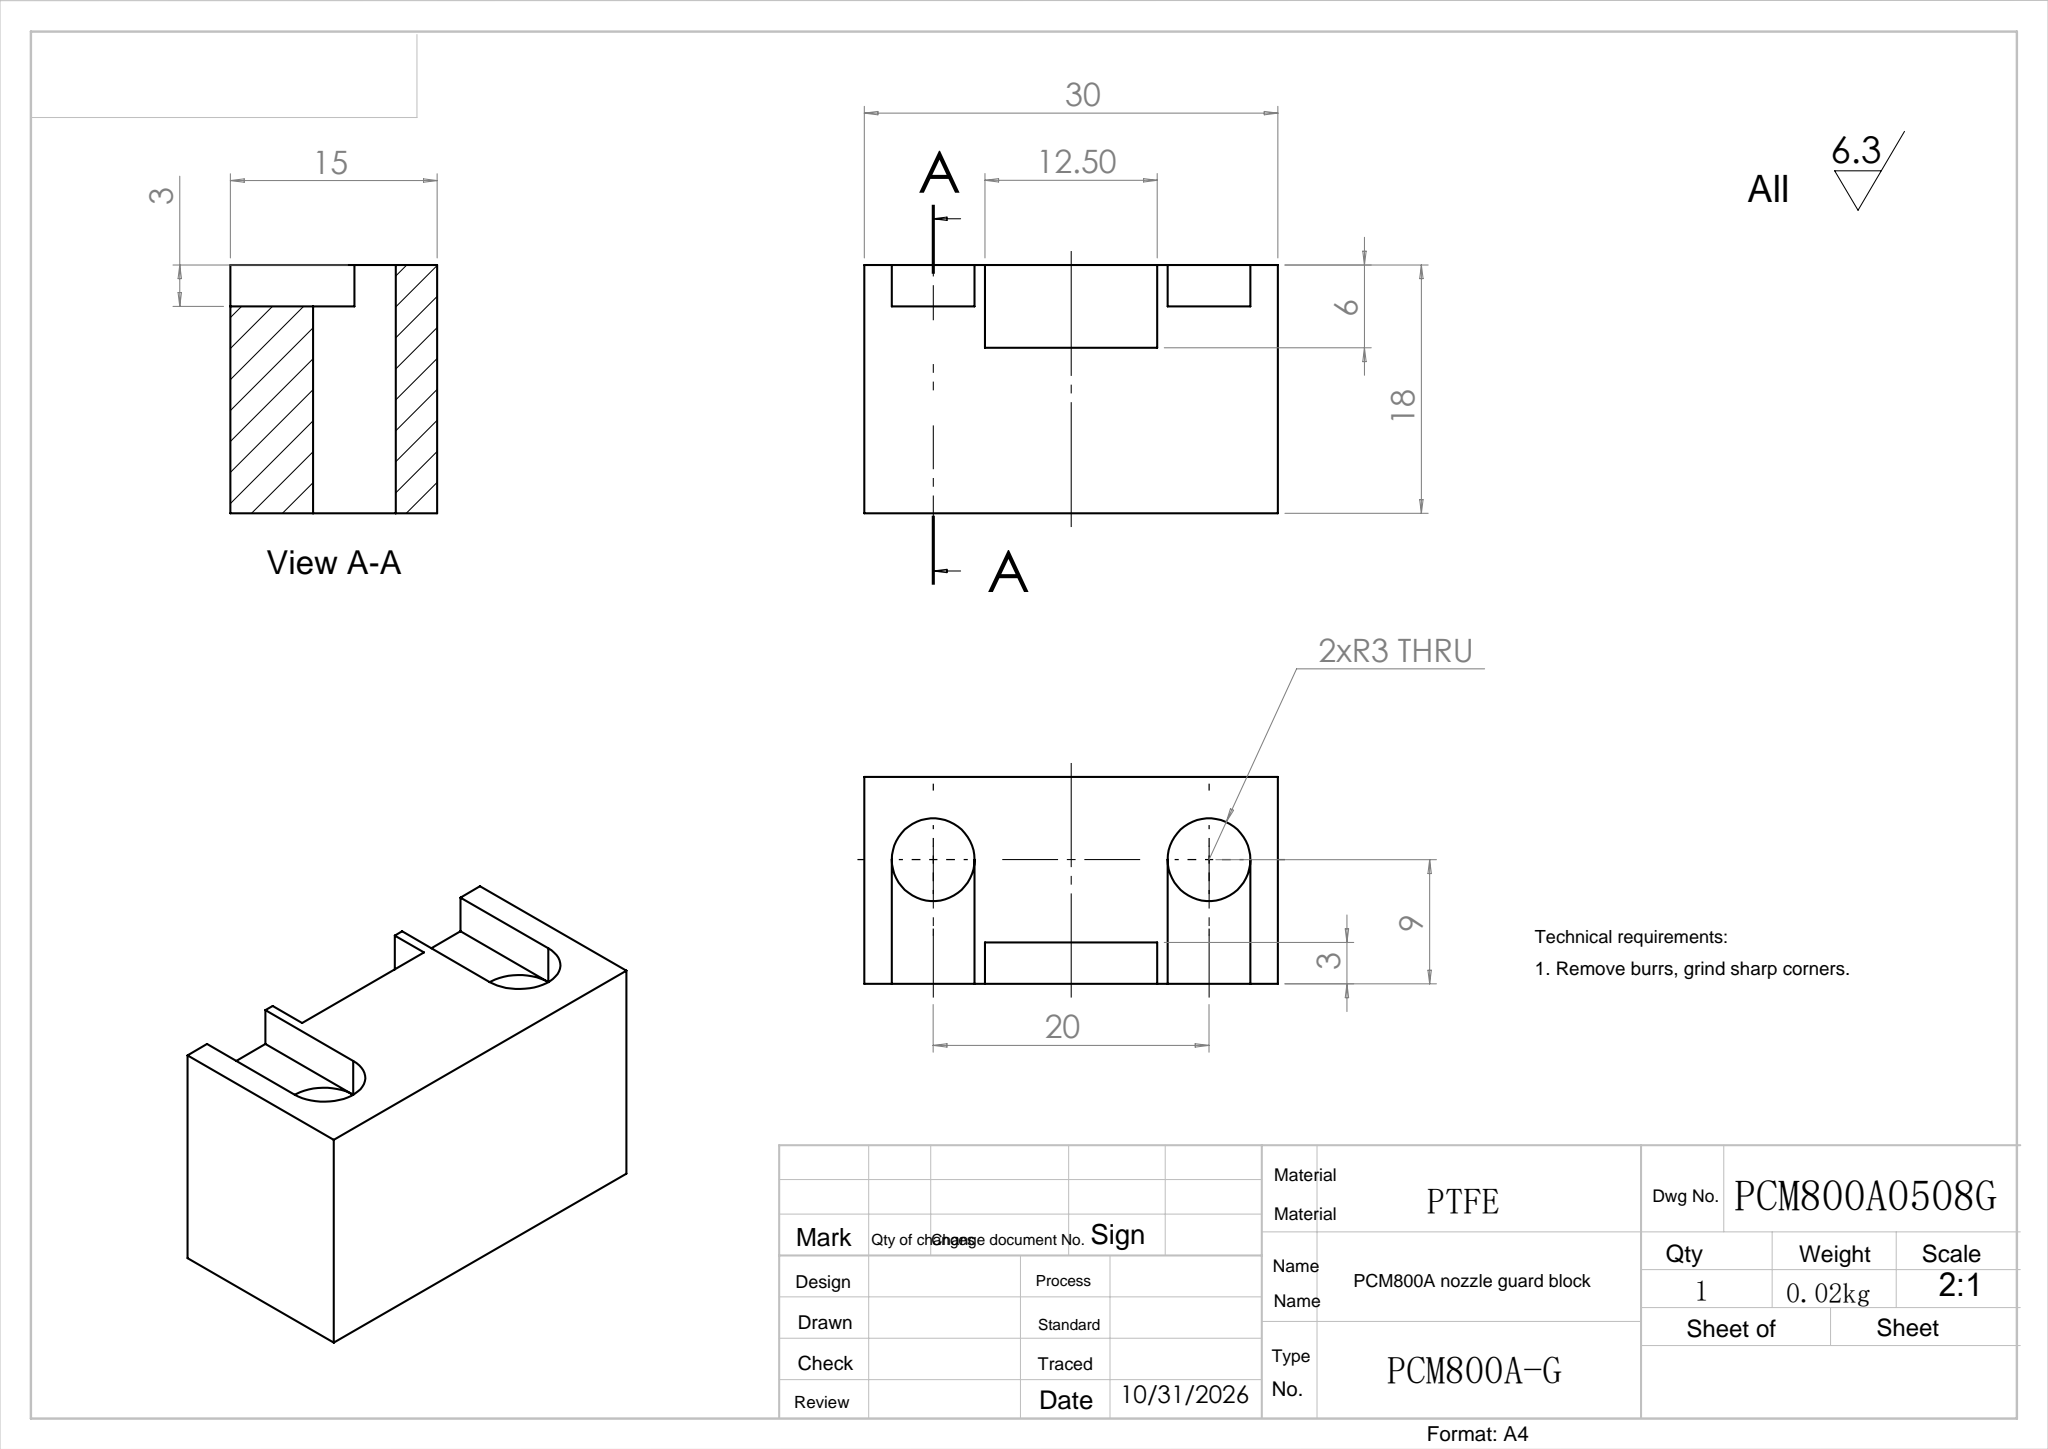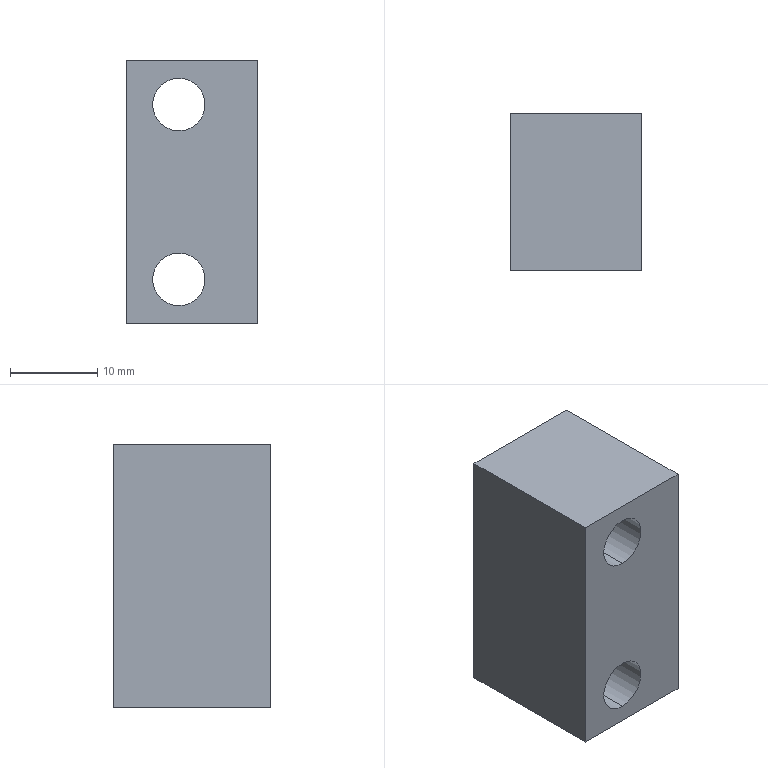Part | SolidWorks | features Cut 3, Extrusion 1, LPattern 1 | 1 solid | 20 faces | box 15 x 18 x 30 mm | volume 6618 mm3 | plane 16 | cylinder 4 | commonest cylinder face diameters 6 x4
STEP:
#1=CARTESIAN_POINT('',(6.,0.,22.));
#2=VERTEX_POINT('',#1);
#3=CARTESIAN_POINT('',(6.,0.,28.));
#4=VERTEX_POINT('',#3);
#5=CARTESIAN_POINT('',(6.,0.,25.));
#6=DIRECTION('',(0.,1.,0.));
#7=DIRECTION('',(0.,0.,1.));
#8=AXIS2_PLACEMENT_3D('',#5,#6,#7);
#9=CIRCLE('',#8,3.);
#10=EDGE_CURVE('',#2,#4,#9,.T.);
#11=ORIENTED_EDGE('',*,*,#10,.F.);
#12=CARTESIAN_POINT('',(6.,15.,22.));
#13=VERTEX_POINT('',#12);
#14=CARTESIAN_POINT('',(6.,0.,22.));
#15=DIRECTION('',(0.,1.,0.));
#16=VECTOR('',#15,1000.);
#17=LINE('',#14,#16);
#18=EDGE_CURVE('',#2,#13,#17,.T.);
#19=ORIENTED_EDGE('',*,*,#18,.T.);
#20=CARTESIAN_POINT('',(6.,18.,22.));
#21=VERTEX_POINT('',#20);
#22=CARTESIAN_POINT('',(6.,15.,22.));
#23=DIRECTION('',(0.,1.,0.));
#24=VECTOR('',#23,1000.);
#25=LINE('',#22,#24);
#26=EDGE_CURVE('',#13,#21,#25,.T.);
#27=ORIENTED_EDGE('',*,*,#26,.T.);
#28=CARTESIAN_POINT('',(6.,18.,28.));
#29=VERTEX_POINT('',#28);
#30=CARTESIAN_POINT('',(6.,18.,25.));
#31=DIRECTION('',(0.,1.,0.));
#32=DIRECTION('',(0.,0.,1.));
#33=AXIS2_PLACEMENT_3D('',#30,#31,#32);
#34=CIRCLE('',#33,3.);
#35=EDGE_CURVE('',#21,#29,#34,.T.);
#36=ORIENTED_EDGE('',*,*,#35,.T.);
#37=CARTESIAN_POINT('',(6.,15.,28.));
#38=VERTEX_POINT('',#37);
#39=CARTESIAN_POINT('',(6.,15.,28.));
#40=DIRECTION('',(0.,1.,0.));
#41=VECTOR('',#40,1000.);
#42=LINE('',#39,#41);
#43=EDGE_CURVE('',#38,#29,#42,.T.);
#44=ORIENTED_EDGE('',*,*,#43,.F.);
#45=CARTESIAN_POINT('',(6.,0.,28.));
#46=DIRECTION('',(0.,1.,0.));
#47=VECTOR('',#46,1000.);
#48=LINE('',#45,#47);
#49=EDGE_CURVE('',#4,#38,#48,.T.);
#50=ORIENTED_EDGE('',*,*,#49,.F.);
#51=EDGE_LOOP('',(#11,#19,#27,#36,#44,#50));
#52=FACE_OUTER_BOUND('',#51,.T.);
#53=CARTESIAN_POINT('',(6.,0.,25.));
#54=DIRECTION('',(0.,1.,0.));
#55=DIRECTION('',(0.,0.,1.));
#56=AXIS2_PLACEMENT_3D('',#53,#54,#55);
#57=CYLINDRICAL_SURFACE('',#56,3.);
#58=ADVANCED_FACE('',(#52),#57,.F.);
#59=CARTESIAN_POINT('',(6.,0.,2.));
#60=VERTEX_POINT('',#59);
#61=CARTESIAN_POINT('',(6.,0.,8.));
#62=VERTEX_POINT('',#61);
#63=CARTESIAN_POINT('',(6.,0.,5.));
#64=DIRECTION('',(0.,1.,0.));
#65=DIRECTION('',(0.,0.,1.));
#66=AXIS2_PLACEMENT_3D('',#63,#64,#65);
#67=CIRCLE('',#66,3.);
#68=EDGE_CURVE('',#60,#62,#67,.T.);
#69=ORIENTED_EDGE('',*,*,#68,.F.);
#70=CARTESIAN_POINT('',(6.,15.,2.));
#71=VERTEX_POINT('',#70);
#72=CARTESIAN_POINT('',(6.,0.,2.));
#73=DIRECTION('',(0.,1.,0.));
#74=VECTOR('',#73,1000.);
#75=LINE('',#72,#74);
#76=EDGE_CURVE('',#60,#71,#75,.T.);
#77=ORIENTED_EDGE('',*,*,#76,.T.);
#78=CARTESIAN_POINT('',(6.,18.,2.));
#79=VERTEX_POINT('',#78);
#80=CARTESIAN_POINT('',(6.,15.,2.));
#81=DIRECTION('',(0.,1.,0.));
#82=VECTOR('',#81,1000.);
#83=LINE('',#80,#82);
#84=EDGE_CURVE('',#71,#79,#83,.T.);
#85=ORIENTED_EDGE('',*,*,#84,.T.);
#86=CARTESIAN_POINT('',(6.,18.,8.));
#87=VERTEX_POINT('',#86);
#88=CARTESIAN_POINT('',(6.,18.,5.));
#89=DIRECTION('',(0.,1.,0.));
#90=DIRECTION('',(0.,0.,1.));
#91=AXIS2_PLACEMENT_3D('',#88,#89,#90);
#92=CIRCLE('',#91,3.);
#93=EDGE_CURVE('',#79,#87,#92,.T.);
#94=ORIENTED_EDGE('',*,*,#93,.T.);
#95=CARTESIAN_POINT('',(6.,15.,8.));
#96=VERTEX_POINT('',#95);
#97=CARTESIAN_POINT('',(6.,15.,8.));
#98=DIRECTION('',(0.,1.,0.));
#99=VECTOR('',#98,1000.);
#100=LINE('',#97,#99);
#101=EDGE_CURVE('',#96,#87,#100,.T.);
#102=ORIENTED_EDGE('',*,*,#101,.F.);
#103=CARTESIAN_POINT('',(6.,0.,8.));
#104=DIRECTION('',(0.,1.,0.));
#105=VECTOR('',#104,1000.);
#106=LINE('',#103,#105);
#107=EDGE_CURVE('',#62,#96,#106,.T.);
#108=ORIENTED_EDGE('',*,*,#107,.F.);
#109=EDGE_LOOP('',(#69,#77,#85,#94,#102,#108));
#110=FACE_OUTER_BOUND('',#109,.T.);
#111=CARTESIAN_POINT('',(6.,0.,5.));
#112=DIRECTION('',(0.,1.,0.));
#113=DIRECTION('',(0.,0.,1.));
#114=AXIS2_PLACEMENT_3D('',#111,#112,#113);
#115=CYLINDRICAL_SURFACE('',#114,3.);
#116=ADVANCED_FACE('',(#110),#115,.F.);
#117=CARTESIAN_POINT('',(15.,12.,21.25));
#118=VERTEX_POINT('',#117);
#119=CARTESIAN_POINT('',(15.,18.,21.25));
#120=VERTEX_POINT('',#119);
#121=CARTESIAN_POINT('',(15.,12.,21.25));
#122=DIRECTION('',(0.,1.,0.));
#123=VECTOR('',#122,1000.);
#124=LINE('',#121,#123);
#125=EDGE_CURVE('',#118,#120,#124,.T.);
#126=ORIENTED_EDGE('',*,*,#125,.T.);
#127=CARTESIAN_POINT('',(15.,18.,22.));
#128=VERTEX_POINT('',#127);
#129=CARTESIAN_POINT('',(15.,18.,30.));
#130=DIRECTION('',(0.,0.,-1.));
#131=VECTOR('',#130,1000.);
#132=LINE('',#129,#131);
#133=EDGE_CURVE('',#128,#120,#132,.T.);
#134=ORIENTED_EDGE('',*,*,#133,.F.);
#135=CARTESIAN_POINT('',(15.,15.,22.));
#136=VERTEX_POINT('',#135);
#137=CARTESIAN_POINT('',(15.,15.,22.));
#138=DIRECTION('',(0.,1.,0.));
#139=VECTOR('',#138,1000.);
#140=LINE('',#137,#139);
#141=EDGE_CURVE('',#136,#128,#140,.T.);
#142=ORIENTED_EDGE('',*,*,#141,.F.);
#143=CARTESIAN_POINT('',(15.,15.,28.));
#144=VERTEX_POINT('',#143);
#145=CARTESIAN_POINT('',(15.,15.,22.));
#146=DIRECTION('',(0.,0.,-1.));
#147=VECTOR('',#146,1000.);
#148=LINE('',#145,#147);
#149=EDGE_CURVE('',#144,#136,#148,.T.);
#150=ORIENTED_EDGE('',*,*,#149,.F.);
#151=CARTESIAN_POINT('',(15.,18.,28.));
#152=VERTEX_POINT('',#151);
#153=CARTESIAN_POINT('',(15.,15.,28.));
#154=DIRECTION('',(0.,1.,0.));
#155=VECTOR('',#154,1000.);
#156=LINE('',#153,#155);
#157=EDGE_CURVE('',#144,#152,#156,.T.);
#158=ORIENTED_EDGE('',*,*,#157,.T.);
#159=CARTESIAN_POINT('',(15.,18.,30.));
#160=VERTEX_POINT('',#159);
#161=CARTESIAN_POINT('',(15.,18.,30.));
#162=DIRECTION('',(0.,0.,-1.));
#163=VECTOR('',#162,1000.);
#164=LINE('',#161,#163);
#165=EDGE_CURVE('',#160,#152,#164,.T.);
#166=ORIENTED_EDGE('',*,*,#165,.F.);
#167=CARTESIAN_POINT('',(15.,0.,30.));
#168=VERTEX_POINT('',#167);
#169=CARTESIAN_POINT('',(15.,0.,30.));
#170=DIRECTION('',(0.,1.,0.));
#171=VECTOR('',#170,1000.);
#172=LINE('',#169,#171);
#173=EDGE_CURVE('',#168,#160,#172,.T.);
#174=ORIENTED_EDGE('',*,*,#173,.F.);
#175=CARTESIAN_POINT('',(15.,0.,0.));
#176=VERTEX_POINT('',#175);
#177=CARTESIAN_POINT('',(15.,0.,30.));
#178=DIRECTION('',(0.,0.,-1.));
#179=VECTOR('',#178,1000.);
#180=LINE('',#177,#179);
#181=EDGE_CURVE('',#168,#176,#180,.T.);
#182=ORIENTED_EDGE('',*,*,#181,.T.);
#183=CARTESIAN_POINT('',(15.,18.,0.));
#184=VERTEX_POINT('',#183);
#185=CARTESIAN_POINT('',(15.,0.,0.));
#186=DIRECTION('',(0.,1.,0.));
#187=VECTOR('',#186,1000.);
#188=LINE('',#185,#187);
#189=EDGE_CURVE('',#176,#184,#188,.T.);
#190=ORIENTED_EDGE('',*,*,#189,.T.);
#191=CARTESIAN_POINT('',(15.,18.,2.));
#192=VERTEX_POINT('',#191);
#193=CARTESIAN_POINT('',(15.,18.,30.));
#194=DIRECTION('',(0.,0.,-1.));
#195=VECTOR('',#194,1000.);
#196=LINE('',#193,#195);
#197=EDGE_CURVE('',#192,#184,#196,.T.);
#198=ORIENTED_EDGE('',*,*,#197,.F.);
#199=CARTESIAN_POINT('',(15.,15.,2.));
#200=VERTEX_POINT('',#199);
#201=CARTESIAN_POINT('',(15.,15.,2.));
#202=DIRECTION('',(0.,1.,0.));
#203=VECTOR('',#202,1000.);
#204=LINE('',#201,#203);
#205=EDGE_CURVE('',#200,#192,#204,.T.);
#206=ORIENTED_EDGE('',*,*,#205,.F.);
#207=CARTESIAN_POINT('',(15.,15.,8.));
#208=VERTEX_POINT('',#207);
#209=CARTESIAN_POINT('',(15.,15.,2.));
#210=DIRECTION('',(0.,0.,-1.));
#211=VECTOR('',#210,1000.);
#212=LINE('',#209,#211);
#213=EDGE_CURVE('',#208,#200,#212,.T.);
#214=ORIENTED_EDGE('',*,*,#213,.F.);
#215=CARTESIAN_POINT('',(15.,18.,8.));
#216=VERTEX_POINT('',#215);
#217=CARTESIAN_POINT('',(15.,15.,8.));
#218=DIRECTION('',(0.,1.,0.));
#219=VECTOR('',#218,1000.);
#220=LINE('',#217,#219);
#221=EDGE_CURVE('',#208,#216,#220,.T.);
#222=ORIENTED_EDGE('',*,*,#221,.T.);
#223=CARTESIAN_POINT('',(15.,18.,8.75));
#224=VERTEX_POINT('',#223);
#225=CARTESIAN_POINT('',(15.,18.,30.));
#226=DIRECTION('',(0.,0.,-1.));
#227=VECTOR('',#226,1000.);
#228=LINE('',#225,#227);
#229=EDGE_CURVE('',#224,#216,#228,.T.);
#230=ORIENTED_EDGE('',*,*,#229,.F.);
#231=CARTESIAN_POINT('',(15.,12.,8.75));
#232=VERTEX_POINT('',#231);
#233=CARTESIAN_POINT('',(15.,12.,8.75));
#234=DIRECTION('',(0.,-1.,0.));
#235=VECTOR('',#234,1000.);
#236=LINE('',#233,#235);
#237=EDGE_CURVE('',#224,#232,#236,.T.);
#238=ORIENTED_EDGE('',*,*,#237,.T.);
#239=CARTESIAN_POINT('',(15.,12.,21.25));
#240=DIRECTION('',(0.,0.,1.));
#241=VECTOR('',#240,1000.);
#242=LINE('',#239,#241);
#243=EDGE_CURVE('',#232,#118,#242,.T.);
#244=ORIENTED_EDGE('',*,*,#243,.T.);
#245=EDGE_LOOP('',(#126,#134,#142,#150,#158,#166,#174,#182,#190,#198,#206,#214,#222,#230,#238,#244));
#246=FACE_OUTER_BOUND('',#245,.T.);
#247=CARTESIAN_POINT('',(15.,0.,30.));
#248=DIRECTION('',(-1.,0.,0.));
#249=DIRECTION('',(0.,0.,1.));
#250=AXIS2_PLACEMENT_3D('',#247,#248,#249);
#251=PLANE('',#250);
#252=ADVANCED_FACE('',(#246),#251,.F.);
#253=CARTESIAN_POINT('',(12.,18.,21.25));
#254=VERTEX_POINT('',#253);
#255=CARTESIAN_POINT('',(12.,18.,21.25));
#256=DIRECTION('',(1.,0.,0.));
#257=VECTOR('',#256,1000.);
#258=LINE('',#255,#257);
#259=EDGE_CURVE('',#254,#120,#258,.T.);
#260=ORIENTED_EDGE('',*,*,#259,.F.);
#261=CARTESIAN_POINT('',(12.,18.,8.75));
#262=VERTEX_POINT('',#261);
#263=CARTESIAN_POINT('',(12.,18.,21.25));
#264=DIRECTION('',(0.,0.,-1.));
#265=VECTOR('',#264,1000.);
#266=LINE('',#263,#265);
#267=EDGE_CURVE('',#254,#262,#266,.T.);
#268=ORIENTED_EDGE('',*,*,#267,.T.);
#269=CARTESIAN_POINT('',(12.,18.,8.75));
#270=DIRECTION('',(1.,0.,0.));
#271=VECTOR('',#270,1000.);
#272=LINE('',#269,#271);
#273=EDGE_CURVE('',#262,#224,#272,.T.);
#274=ORIENTED_EDGE('',*,*,#273,.T.);
#275=ORIENTED_EDGE('',*,*,#229,.T.);
#276=CARTESIAN_POINT('',(15.,18.,8.));
#277=DIRECTION('',(1.,0.,0.));
#278=VECTOR('',#277,1000.);
#279=LINE('',#276,#278);
#280=EDGE_CURVE('',#87,#216,#279,.T.);
#281=ORIENTED_EDGE('',*,*,#280,.F.);
#282=ORIENTED_EDGE('',*,*,#93,.F.);
#283=CARTESIAN_POINT('',(15.,18.,2.));
#284=DIRECTION('',(-1.,0.,0.));
#285=VECTOR('',#284,1000.);
#286=LINE('',#283,#285);
#287=EDGE_CURVE('',#192,#79,#286,.T.);
#288=ORIENTED_EDGE('',*,*,#287,.F.);
#289=ORIENTED_EDGE('',*,*,#197,.T.);
#290=CARTESIAN_POINT('',(0.,18.,0.));
#291=VERTEX_POINT('',#290);
#292=CARTESIAN_POINT('',(0.,18.,0.));
#293=DIRECTION('',(-1.,0.,0.));
#294=VECTOR('',#293,1000.);
#295=LINE('',#292,#294);
#296=EDGE_CURVE('',#184,#291,#295,.T.);
#297=ORIENTED_EDGE('',*,*,#296,.T.);
#298=CARTESIAN_POINT('',(0.,18.,30.));
#299=VERTEX_POINT('',#298);
#300=CARTESIAN_POINT('',(0.,18.,30.));
#301=DIRECTION('',(0.,0.,-1.));
#302=VECTOR('',#301,1000.);
#303=LINE('',#300,#302);
#304=EDGE_CURVE('',#299,#291,#303,.T.);
#305=ORIENTED_EDGE('',*,*,#304,.F.);
#306=CARTESIAN_POINT('',(0.,18.,30.));
#307=DIRECTION('',(-1.,0.,0.));
#308=VECTOR('',#307,1000.);
#309=LINE('',#306,#308);
#310=EDGE_CURVE('',#160,#299,#309,.T.);
#311=ORIENTED_EDGE('',*,*,#310,.F.);
#312=ORIENTED_EDGE('',*,*,#165,.T.);
#313=CARTESIAN_POINT('',(15.,18.,28.));
#314=DIRECTION('',(1.,0.,0.));
#315=VECTOR('',#314,1000.);
#316=LINE('',#313,#315);
#317=EDGE_CURVE('',#29,#152,#316,.T.);
#318=ORIENTED_EDGE('',*,*,#317,.F.);
#319=ORIENTED_EDGE('',*,*,#35,.F.);
#320=CARTESIAN_POINT('',(15.,18.,22.));
#321=DIRECTION('',(-1.,0.,0.));
#322=VECTOR('',#321,1000.);
#323=LINE('',#320,#322);
#324=EDGE_CURVE('',#128,#21,#323,.T.);
#325=ORIENTED_EDGE('',*,*,#324,.F.);
#326=ORIENTED_EDGE('',*,*,#133,.T.);
#327=EDGE_LOOP('',(#260,#268,#274,#275,#281,#282,#288,#289,#297,#305,#311,#312,#318,#319,#325,#326));
#328=FACE_OUTER_BOUND('',#327,.T.);
#329=CARTESIAN_POINT('',(0.,18.,30.));
#330=DIRECTION('',(0.,-1.,0.));
#331=DIRECTION('',(0.,0.,-1.));
#332=AXIS2_PLACEMENT_3D('',#329,#330,#331);
#333=PLANE('',#332);
#334=ADVANCED_FACE('',(#328),#333,.F.);
#335=CARTESIAN_POINT('',(0.,0.,0.));
#336=VERTEX_POINT('',#335);
#337=CARTESIAN_POINT('',(0.,0.,0.));
#338=DIRECTION('',(0.,-1.,0.));
#339=VECTOR('',#338,1000.);
#340=LINE('',#337,#339);
#341=EDGE_CURVE('',#291,#336,#340,.T.);
#342=ORIENTED_EDGE('',*,*,#341,.T.);
#343=CARTESIAN_POINT('',(0.,0.,30.));
#344=VERTEX_POINT('',#343);
#345=CARTESIAN_POINT('',(0.,0.,30.));
#346=DIRECTION('',(0.,0.,-1.));
#347=VECTOR('',#346,1000.);
#348=LINE('',#345,#347);
#349=EDGE_CURVE('',#344,#336,#348,.T.);
#350=ORIENTED_EDGE('',*,*,#349,.F.);
#351=CARTESIAN_POINT('',(0.,0.,30.));
#352=DIRECTION('',(0.,-1.,0.));
#353=VECTOR('',#352,1000.);
#354=LINE('',#351,#353);
#355=EDGE_CURVE('',#299,#344,#354,.T.);
#356=ORIENTED_EDGE('',*,*,#355,.F.);
#357=ORIENTED_EDGE('',*,*,#304,.T.);
#358=EDGE_LOOP('',(#342,#350,#356,#357));
#359=FACE_OUTER_BOUND('',#358,.T.);
#360=CARTESIAN_POINT('',(0.,0.,30.));
#361=DIRECTION('',(1.,0.,0.));
#362=DIRECTION('',(0.,0.,-1.));
#363=AXIS2_PLACEMENT_3D('',#360,#361,#362);
#364=PLANE('',#363);
#365=ADVANCED_FACE('',(#359),#364,.F.);
#366=CARTESIAN_POINT('',(6.,0.,25.));
#367=DIRECTION('',(0.,1.,0.));
#368=DIRECTION('',(0.,0.,1.));
#369=AXIS2_PLACEMENT_3D('',#366,#367,#368);
#370=CIRCLE('',#369,3.);
#371=EDGE_CURVE('',#4,#2,#370,.T.);
#372=ORIENTED_EDGE('',*,*,#371,.T.);
#373=ORIENTED_EDGE('',*,*,#10,.T.);
#374=EDGE_LOOP('',(#372,#373));
#375=FACE_BOUND('',#374,.T.);
#376=CARTESIAN_POINT('',(6.,0.,5.));
#377=DIRECTION('',(0.,1.,0.));
#378=DIRECTION('',(0.,0.,1.));
#379=AXIS2_PLACEMENT_3D('',#376,#377,#378);
#380=CIRCLE('',#379,3.);
#381=EDGE_CURVE('',#62,#60,#380,.T.);
#382=ORIENTED_EDGE('',*,*,#381,.T.);
#383=ORIENTED_EDGE('',*,*,#68,.T.);
#384=EDGE_LOOP('',(#382,#383));
#385=FACE_BOUND('',#384,.T.);
#386=CARTESIAN_POINT('',(0.,0.,0.));
#387=DIRECTION('',(1.,0.,0.));
#388=VECTOR('',#387,1000.);
#389=LINE('',#386,#388);
#390=EDGE_CURVE('',#336,#176,#389,.T.);
#391=ORIENTED_EDGE('',*,*,#390,.T.);
#392=ORIENTED_EDGE('',*,*,#181,.F.);
#393=CARTESIAN_POINT('',(0.,0.,30.));
#394=DIRECTION('',(1.,0.,0.));
#395=VECTOR('',#394,1000.);
#396=LINE('',#393,#395);
#397=EDGE_CURVE('',#344,#168,#396,.T.);
#398=ORIENTED_EDGE('',*,*,#397,.F.);
#399=ORIENTED_EDGE('',*,*,#349,.T.);
#400=EDGE_LOOP('',(#391,#392,#398,#399));
#401=FACE_OUTER_BOUND('',#400,.T.);
#402=CARTESIAN_POINT('',(0.,0.,30.));
#403=DIRECTION('',(0.,1.,0.));
#404=DIRECTION('',(0.,0.,1.));
#405=AXIS2_PLACEMENT_3D('',#402,#403,#404);
#406=PLANE('',#405);
#407=ADVANCED_FACE('',(#375,#385,#401),#406,.F.);
#408=ORIENTED_EDGE('',*,*,#355,.T.);
#409=ORIENTED_EDGE('',*,*,#397,.T.);
#410=ORIENTED_EDGE('',*,*,#173,.T.);
#411=ORIENTED_EDGE('',*,*,#310,.T.);
#412=EDGE_LOOP('',(#408,#409,#410,#411));
#413=FACE_OUTER_BOUND('',#412,.T.);
#414=CARTESIAN_POINT('',(0.,18.,30.));
#415=DIRECTION('',(0.,0.,-1.));
#416=DIRECTION('',(-1.,0.,0.));
#417=AXIS2_PLACEMENT_3D('',#414,#415,#416);
#418=PLANE('',#417);
#419=ADVANCED_FACE('',(#413),#418,.F.);
#420=ORIENTED_EDGE('',*,*,#341,.F.);
#421=ORIENTED_EDGE('',*,*,#296,.F.);
#422=ORIENTED_EDGE('',*,*,#189,.F.);
#423=ORIENTED_EDGE('',*,*,#390,.F.);
#424=EDGE_LOOP('',(#420,#421,#422,#423));
#425=FACE_OUTER_BOUND('',#424,.T.);
#426=CARTESIAN_POINT('',(0.,18.,0.));
#427=DIRECTION('',(0.,0.,-1.));
#428=DIRECTION('',(-1.,0.,0.));
#429=AXIS2_PLACEMENT_3D('',#426,#427,#428);
#430=PLANE('',#429);
#431=ADVANCED_FACE('',(#425),#430,.T.);
#432=ORIENTED_EDGE('',*,*,#76,.F.);
#433=ORIENTED_EDGE('',*,*,#381,.F.);
#434=ORIENTED_EDGE('',*,*,#107,.T.);
#435=CARTESIAN_POINT('',(6.,15.,5.));
#436=DIRECTION('',(0.,-1.,0.));
#437=DIRECTION('',(0.,0.,1.));
#438=AXIS2_PLACEMENT_3D('',#435,#436,#437);
#439=CIRCLE('',#438,3.);
#440=EDGE_CURVE('',#71,#96,#439,.T.);
#441=ORIENTED_EDGE('',*,*,#440,.F.);
#442=EDGE_LOOP('',(#432,#433,#434,#441));
#443=FACE_OUTER_BOUND('',#442,.T.);
#444=CARTESIAN_POINT('',(6.,0.,5.));
#445=DIRECTION('',(0.,1.,0.));
#446=DIRECTION('',(0.,0.,1.));
#447=AXIS2_PLACEMENT_3D('',#444,#445,#446);
#448=CYLINDRICAL_SURFACE('',#447,3.);
#449=ADVANCED_FACE('',(#443),#448,.F.);
#450=ORIENTED_EDGE('',*,*,#440,.T.);
#451=CARTESIAN_POINT('',(15.,15.,8.));
#452=DIRECTION('',(1.,0.,0.));
#453=VECTOR('',#452,1000.);
#454=LINE('',#451,#453);
#455=EDGE_CURVE('',#96,#208,#454,.T.);
#456=ORIENTED_EDGE('',*,*,#455,.T.);
#457=ORIENTED_EDGE('',*,*,#213,.T.);
#458=CARTESIAN_POINT('',(15.,15.,2.));
#459=DIRECTION('',(-1.,0.,0.));
#460=VECTOR('',#459,1000.);
#461=LINE('',#458,#460);
#462=EDGE_CURVE('',#200,#71,#461,.T.);
#463=ORIENTED_EDGE('',*,*,#462,.T.);
#464=EDGE_LOOP('',(#450,#456,#457,#463));
#465=FACE_OUTER_BOUND('',#464,.T.);
#466=CARTESIAN_POINT('',(6.,15.,5.));
#467=DIRECTION('',(0.,1.,0.));
#468=DIRECTION('',(0.,0.,1.));
#469=AXIS2_PLACEMENT_3D('',#466,#467,#468);
#470=PLANE('',#469);
#471=ADVANCED_FACE('',(#465),#470,.T.);
#472=ORIENTED_EDGE('',*,*,#280,.T.);
#473=ORIENTED_EDGE('',*,*,#221,.F.);
#474=ORIENTED_EDGE('',*,*,#455,.F.);
#475=ORIENTED_EDGE('',*,*,#101,.T.);
#476=EDGE_LOOP('',(#472,#473,#474,#475));
#477=FACE_OUTER_BOUND('',#476,.T.);
#478=CARTESIAN_POINT('',(15.,15.,8.));
#479=DIRECTION('',(0.,0.,1.));
#480=DIRECTION('',(1.,0.,0.));
#481=AXIS2_PLACEMENT_3D('',#478,#479,#480);
#482=PLANE('',#481);
#483=ADVANCED_FACE('',(#477),#482,.F.);
#484=ORIENTED_EDGE('',*,*,#287,.T.);
#485=ORIENTED_EDGE('',*,*,#84,.F.);
#486=ORIENTED_EDGE('',*,*,#462,.F.);
#487=ORIENTED_EDGE('',*,*,#205,.T.);
#488=EDGE_LOOP('',(#484,#485,#486,#487));
#489=FACE_OUTER_BOUND('',#488,.T.);
#490=CARTESIAN_POINT('',(15.,15.,2.));
#491=DIRECTION('',(0.,0.,-1.));
#492=DIRECTION('',(-1.,0.,0.));
#493=AXIS2_PLACEMENT_3D('',#490,#491,#492);
#494=PLANE('',#493);
#495=ADVANCED_FACE('',(#489),#494,.F.);
#496=ORIENTED_EDGE('',*,*,#18,.F.);
#497=ORIENTED_EDGE('',*,*,#371,.F.);
#498=ORIENTED_EDGE('',*,*,#49,.T.);
#499=CARTESIAN_POINT('',(6.,15.,25.));
#500=DIRECTION('',(0.,-1.,0.));
#501=DIRECTION('',(0.,0.,1.));
#502=AXIS2_PLACEMENT_3D('',#499,#500,#501);
#503=CIRCLE('',#502,3.);
#504=EDGE_CURVE('',#13,#38,#503,.T.);
#505=ORIENTED_EDGE('',*,*,#504,.F.);
#506=EDGE_LOOP('',(#496,#497,#498,#505));
#507=FACE_OUTER_BOUND('',#506,.T.);
#508=CARTESIAN_POINT('',(6.,0.,25.));
#509=DIRECTION('',(0.,1.,0.));
#510=DIRECTION('',(0.,0.,1.));
#511=AXIS2_PLACEMENT_3D('',#508,#509,#510);
#512=CYLINDRICAL_SURFACE('',#511,3.);
#513=ADVANCED_FACE('',(#507),#512,.F.);
#514=ORIENTED_EDGE('',*,*,#504,.T.);
#515=CARTESIAN_POINT('',(15.,15.,28.));
#516=DIRECTION('',(1.,0.,0.));
#517=VECTOR('',#516,1000.);
#518=LINE('',#515,#517);
#519=EDGE_CURVE('',#38,#144,#518,.T.);
#520=ORIENTED_EDGE('',*,*,#519,.T.);
#521=ORIENTED_EDGE('',*,*,#149,.T.);
#522=CARTESIAN_POINT('',(15.,15.,22.));
#523=DIRECTION('',(-1.,0.,0.));
#524=VECTOR('',#523,1000.);
#525=LINE('',#522,#524);
#526=EDGE_CURVE('',#136,#13,#525,.T.);
#527=ORIENTED_EDGE('',*,*,#526,.T.);
#528=EDGE_LOOP('',(#514,#520,#521,#527));
#529=FACE_OUTER_BOUND('',#528,.T.);
#530=CARTESIAN_POINT('',(6.,15.,25.));
#531=DIRECTION('',(0.,1.,0.));
#532=DIRECTION('',(0.,0.,1.));
#533=AXIS2_PLACEMENT_3D('',#530,#531,#532);
#534=PLANE('',#533);
#535=ADVANCED_FACE('',(#529),#534,.T.);
#536=ORIENTED_EDGE('',*,*,#317,.T.);
#537=ORIENTED_EDGE('',*,*,#157,.F.);
#538=ORIENTED_EDGE('',*,*,#519,.F.);
#539=ORIENTED_EDGE('',*,*,#43,.T.);
#540=EDGE_LOOP('',(#536,#537,#538,#539));
#541=FACE_OUTER_BOUND('',#540,.T.);
#542=CARTESIAN_POINT('',(15.,15.,28.));
#543=DIRECTION('',(0.,0.,1.));
#544=DIRECTION('',(1.,0.,0.));
#545=AXIS2_PLACEMENT_3D('',#542,#543,#544);
#546=PLANE('',#545);
#547=ADVANCED_FACE('',(#541),#546,.F.);
#548=ORIENTED_EDGE('',*,*,#324,.T.);
#549=ORIENTED_EDGE('',*,*,#26,.F.);
#550=ORIENTED_EDGE('',*,*,#526,.F.);
#551=ORIENTED_EDGE('',*,*,#141,.T.);
#552=EDGE_LOOP('',(#548,#549,#550,#551));
#553=FACE_OUTER_BOUND('',#552,.T.);
#554=CARTESIAN_POINT('',(15.,15.,22.));
#555=DIRECTION('',(0.,0.,-1.));
#556=DIRECTION('',(-1.,0.,0.));
#557=AXIS2_PLACEMENT_3D('',#554,#555,#556);
#558=PLANE('',#557);
#559=ADVANCED_FACE('',(#553),#558,.F.);
#560=ORIENTED_EDGE('',*,*,#243,.F.);
#561=CARTESIAN_POINT('',(12.,12.,8.75));
#562=VERTEX_POINT('',#561);
#563=CARTESIAN_POINT('',(12.,12.,8.75));
#564=DIRECTION('',(1.,0.,0.));
#565=VECTOR('',#564,1000.);
#566=LINE('',#563,#565);
#567=EDGE_CURVE('',#562,#232,#566,.T.);
#568=ORIENTED_EDGE('',*,*,#567,.F.);
#569=CARTESIAN_POINT('',(12.,12.,21.25));
#570=VERTEX_POINT('',#569);
#571=CARTESIAN_POINT('',(12.,12.,21.25));
#572=DIRECTION('',(0.,0.,1.));
#573=VECTOR('',#572,1000.);
#574=LINE('',#571,#573);
#575=EDGE_CURVE('',#562,#570,#574,.T.);
#576=ORIENTED_EDGE('',*,*,#575,.T.);
#577=CARTESIAN_POINT('',(12.,12.,21.25));
#578=DIRECTION('',(1.,0.,0.));
#579=VECTOR('',#578,1000.);
#580=LINE('',#577,#579);
#581=EDGE_CURVE('',#570,#118,#580,.T.);
#582=ORIENTED_EDGE('',*,*,#581,.T.);
#583=EDGE_LOOP('',(#560,#568,#576,#582));
#584=FACE_OUTER_BOUND('',#583,.T.);
#585=CARTESIAN_POINT('',(12.,12.,21.25));
#586=DIRECTION('',(0.,1.,0.));
#587=DIRECTION('',(0.,0.,1.));
#588=AXIS2_PLACEMENT_3D('',#585,#586,#587);
#589=PLANE('',#588);
#590=ADVANCED_FACE('',(#584),#589,.T.);
#591=ORIENTED_EDGE('',*,*,#125,.F.);
#592=ORIENTED_EDGE('',*,*,#581,.F.);
#593=CARTESIAN_POINT('',(12.,12.,21.25));
#594=DIRECTION('',(0.,1.,0.));
#595=VECTOR('',#594,1000.);
#596=LINE('',#593,#595);
#597=EDGE_CURVE('',#570,#254,#596,.T.);
#598=ORIENTED_EDGE('',*,*,#597,.T.);
#599=ORIENTED_EDGE('',*,*,#259,.T.);
#600=EDGE_LOOP('',(#591,#592,#598,#599));
#601=FACE_OUTER_BOUND('',#600,.T.);
#602=CARTESIAN_POINT('',(12.,12.,21.25));
#603=DIRECTION('',(0.,0.,-1.));
#604=DIRECTION('',(-1.,0.,0.));
#605=AXIS2_PLACEMENT_3D('',#602,#603,#604);
#606=PLANE('',#605);
#607=ADVANCED_FACE('',(#601),#606,.T.);
#608=ORIENTED_EDGE('',*,*,#237,.F.);
#609=ORIENTED_EDGE('',*,*,#273,.F.);
#610=CARTESIAN_POINT('',(12.,12.,8.75));
#611=DIRECTION('',(0.,-1.,0.));
#612=VECTOR('',#611,1000.);
#613=LINE('',#610,#612);
#614=EDGE_CURVE('',#262,#562,#613,.T.);
#615=ORIENTED_EDGE('',*,*,#614,.T.);
#616=ORIENTED_EDGE('',*,*,#567,.T.);
#617=EDGE_LOOP('',(#608,#609,#615,#616));
#618=FACE_OUTER_BOUND('',#617,.T.);
#619=CARTESIAN_POINT('',(12.,12.,8.75));
#620=DIRECTION('',(0.,0.,1.));
#621=DIRECTION('',(1.,0.,0.));
#622=AXIS2_PLACEMENT_3D('',#619,#620,#621);
#623=PLANE('',#622);
#624=ADVANCED_FACE('',(#618),#623,.T.);
#625=ORIENTED_EDGE('',*,*,#575,.F.);
#626=ORIENTED_EDGE('',*,*,#614,.F.);
#627=ORIENTED_EDGE('',*,*,#267,.F.);
#628=ORIENTED_EDGE('',*,*,#597,.F.);
#629=EDGE_LOOP('',(#625,#626,#627,#628));
#630=FACE_OUTER_BOUND('',#629,.T.);
#631=CARTESIAN_POINT('',(12.,12.,8.75));
#632=DIRECTION('',(1.,0.,0.));
#633=DIRECTION('',(0.,0.,-1.));
#634=AXIS2_PLACEMENT_3D('',#631,#632,#633);
#635=PLANE('',#634);
#636=ADVANCED_FACE('',(#630),#635,.T.);
#637=CLOSED_SHELL('',(#58,#116,#252,#334,#365,#407,#419,#431,#449,#471,#483,#495,#513,#535,#547,#559,#590,#607,#624,#636));
#638=MANIFOLD_SOLID_BREP('',#637);
#639=CARTESIAN_POINT('',(0.,0.,0.));
#640=DIRECTION('',(0.,0.,1.));
#641=DIRECTION('',(1.,0.,0.));
#642=AXIS2_PLACEMENT_3D('',#639,#640,#641);
#643=(LENGTH_UNIT()NAMED_UNIT(*)SI_UNIT(.MILLI.,.METRE.));
#644=UNCERTAINTY_MEASURE_WITH_UNIT(LENGTH_MEASURE(0.00001),#643,'','');
#645=(NAMED_UNIT(*)PLANE_ANGLE_UNIT()SI_UNIT($,.RADIAN.));
#646=(NAMED_UNIT(*)SI_UNIT($,.STERADIAN.)SOLID_ANGLE_UNIT());
#647=(GEOMETRIC_REPRESENTATION_CONTEXT(3)GLOBAL_UNCERTAINTY_ASSIGNED_CONTEXT((#644))GLOBAL_UNIT_ASSIGNED_CONTEXT((#643,#645,#646))REPRESENTATION_CONTEXT('',''));
#648=ADVANCED_BREP_SHAPE_REPRESENTATION('',(#638,#642),#647);